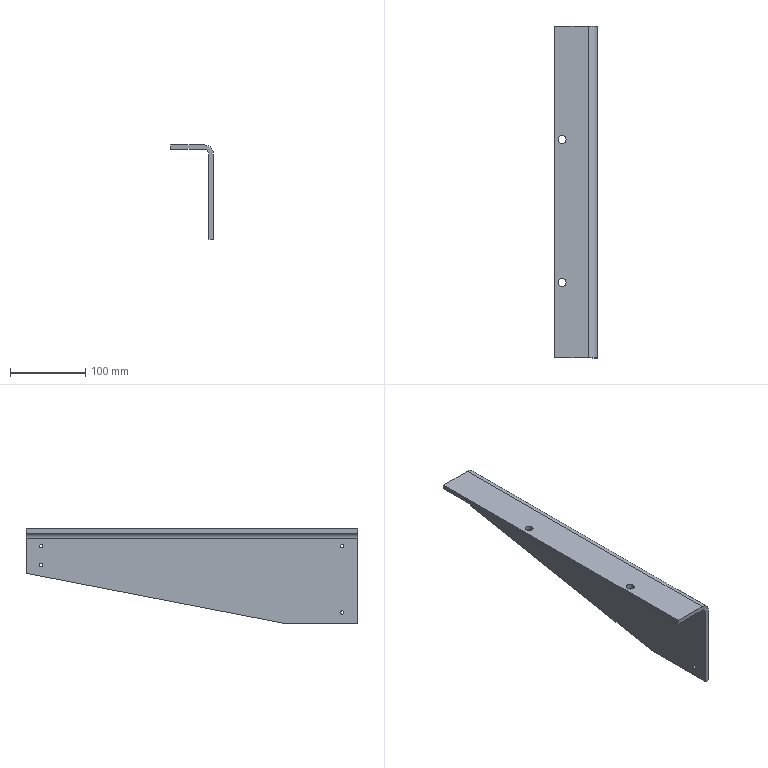Part | NX | features solid 2 | 1 solid | 23 faces | box 57 x 441 x 125 mm | volume 386523 mm3 | cylinder 14 | plane 9 | commonest cylinder face diameters 4.459 x8 10.6 x4 12 x1 24 x1
STEP:
#1=CARTESIAN_POINT('',(-333.,473.229,-255.));
#2=VERTEX_POINT('',#1);
#3=CARTESIAN_POINT('',(-339.,473.229,-255.));
#4=VERTEX_POINT('',#3);
#5=CARTESIAN_POINT('',(-794.904,473.229,-255.));
#6=DIRECTION('',(1.,0.,0.));
#7=VECTOR('',#6,1000.);
#8=LINE('',#5,#7);
#9=EDGE_CURVE('',#2,#4,#8,.F.);
#10=ORIENTED_EDGE('',*,*,#9,.T.);
#11=CARTESIAN_POINT('',(-339.,468.77,-255.));
#12=VERTEX_POINT('',#11);
#13=CARTESIAN_POINT('',(-339.,471.,-255.));
#14=DIRECTION('',(1.,0.,0.));
#15=DIRECTION('',(0.,1.,0.));
#16=AXIS2_PLACEMENT_3D('',#13,#14,#15);
#17=CIRCLE('',#16,2.229);
#18=EDGE_CURVE('',#12,#4,#17,.T.);
#19=ORIENTED_EDGE('',*,*,#18,.F.);
#20=CARTESIAN_POINT('',(-333.,468.77,-255.));
#21=VERTEX_POINT('',#20);
#22=CARTESIAN_POINT('',(-794.904,468.77,-255.));
#23=DIRECTION('',(1.,0.,0.));
#24=VECTOR('',#23,1000.);
#25=LINE('',#22,#24);
#26=EDGE_CURVE('',#12,#21,#25,.T.);
#27=ORIENTED_EDGE('',*,*,#26,.T.);
#28=CARTESIAN_POINT('',(-333.,471.,-255.));
#29=DIRECTION('',(-1.,0.,0.));
#30=DIRECTION('',(0.,-1.,0.));
#31=AXIS2_PLACEMENT_3D('',#28,#29,#30);
#32=CIRCLE('',#31,2.229);
#33=EDGE_CURVE('',#2,#21,#32,.T.);
#34=ORIENTED_EDGE('',*,*,#33,.F.);
#35=EDGE_LOOP('',(#10,#19,#27,#34));
#36=FACE_BOUND('',#35,.T.);
#37=CARTESIAN_POINT('',(-794.904,471.,-255.));
#38=DIRECTION('',(1.,0.,0.));
#39=DIRECTION('',(0.,-1.,0.));
#40=AXIS2_PLACEMENT_3D('',#37,#38,#39);
#41=CYLINDRICAL_SURFACE('',#40,2.229);
#42=ADVANCED_FACE('',(#36),#41,.F.);
#43=CARTESIAN_POINT('',(-333.,473.229,-230.));
#44=VERTEX_POINT('',#43);
#45=CARTESIAN_POINT('',(-339.,473.229,-230.));
#46=VERTEX_POINT('',#45);
#47=CARTESIAN_POINT('',(-794.904,473.229,-230.));
#48=DIRECTION('',(1.,0.,0.));
#49=VECTOR('',#48,1000.);
#50=LINE('',#47,#49);
#51=EDGE_CURVE('',#44,#46,#50,.F.);
#52=ORIENTED_EDGE('',*,*,#51,.T.);
#53=CARTESIAN_POINT('',(-339.,468.77,-230.));
#54=VERTEX_POINT('',#53);
#55=CARTESIAN_POINT('',(-339.,471.,-230.));
#56=DIRECTION('',(1.,0.,0.));
#57=DIRECTION('',(0.,1.,0.));
#58=AXIS2_PLACEMENT_3D('',#55,#56,#57);
#59=CIRCLE('',#58,2.229);
#60=EDGE_CURVE('',#54,#46,#59,.T.);
#61=ORIENTED_EDGE('',*,*,#60,.F.);
#62=CARTESIAN_POINT('',(-333.,468.77,-230.));
#63=VERTEX_POINT('',#62);
#64=CARTESIAN_POINT('',(-794.904,468.77,-230.));
#65=DIRECTION('',(1.,0.,0.));
#66=VECTOR('',#65,1000.);
#67=LINE('',#64,#66);
#68=EDGE_CURVE('',#54,#63,#67,.T.);
#69=ORIENTED_EDGE('',*,*,#68,.T.);
#70=CARTESIAN_POINT('',(-333.,471.,-230.));
#71=DIRECTION('',(-1.,0.,0.));
#72=DIRECTION('',(0.,-1.,0.));
#73=AXIS2_PLACEMENT_3D('',#70,#71,#72);
#74=CIRCLE('',#73,2.229);
#75=EDGE_CURVE('',#44,#63,#74,.T.);
#76=ORIENTED_EDGE('',*,*,#75,.F.);
#77=EDGE_LOOP('',(#52,#61,#69,#76));
#78=FACE_BOUND('',#77,.T.);
#79=CARTESIAN_POINT('',(-794.904,471.,-230.));
#80=DIRECTION('',(1.,0.,0.));
#81=DIRECTION('',(0.,-1.,0.));
#82=AXIS2_PLACEMENT_3D('',#79,#80,#81);
#83=CYLINDRICAL_SURFACE('',#82,2.229);
#84=ADVANCED_FACE('',(#78),#83,.F.);
#85=CARTESIAN_POINT('',(-333.,73.23,-318.));
#86=VERTEX_POINT('',#85);
#87=CARTESIAN_POINT('',(-339.,73.23,-318.));
#88=VERTEX_POINT('',#87);
#89=CARTESIAN_POINT('',(-794.904,73.23,-318.));
#90=DIRECTION('',(1.,0.,0.));
#91=VECTOR('',#90,1000.);
#92=LINE('',#89,#91);
#93=EDGE_CURVE('',#86,#88,#92,.F.);
#94=ORIENTED_EDGE('',*,*,#93,.T.);
#95=CARTESIAN_POINT('',(-339.,68.771,-318.));
#96=VERTEX_POINT('',#95);
#97=CARTESIAN_POINT('',(-339.,71.,-318.));
#98=DIRECTION('',(1.,0.,0.));
#99=DIRECTION('',(0.,1.,0.));
#100=AXIS2_PLACEMENT_3D('',#97,#98,#99);
#101=CIRCLE('',#100,2.229);
#102=EDGE_CURVE('',#96,#88,#101,.T.);
#103=ORIENTED_EDGE('',*,*,#102,.F.);
#104=CARTESIAN_POINT('',(-333.,68.771,-318.));
#105=VERTEX_POINT('',#104);
#106=CARTESIAN_POINT('',(-794.904,68.771,-318.));
#107=DIRECTION('',(1.,0.,0.));
#108=VECTOR('',#107,1000.);
#109=LINE('',#106,#108);
#110=EDGE_CURVE('',#96,#105,#109,.T.);
#111=ORIENTED_EDGE('',*,*,#110,.T.);
#112=CARTESIAN_POINT('',(-333.,71.,-318.));
#113=DIRECTION('',(-1.,0.,0.));
#114=DIRECTION('',(0.,-1.,0.));
#115=AXIS2_PLACEMENT_3D('',#112,#113,#114);
#116=CIRCLE('',#115,2.229);
#117=EDGE_CURVE('',#86,#105,#116,.T.);
#118=ORIENTED_EDGE('',*,*,#117,.F.);
#119=EDGE_LOOP('',(#94,#103,#111,#118));
#120=FACE_BOUND('',#119,.T.);
#121=CARTESIAN_POINT('',(-794.904,71.,-318.));
#122=DIRECTION('',(1.,0.,0.));
#123=DIRECTION('',(0.,-1.,0.));
#124=AXIS2_PLACEMENT_3D('',#121,#122,#123);
#125=CYLINDRICAL_SURFACE('',#124,2.229);
#126=ADVANCED_FACE('',(#120),#125,.F.);
#127=CARTESIAN_POINT('',(-333.,73.23,-230.));
#128=VERTEX_POINT('',#127);
#129=CARTESIAN_POINT('',(-339.,73.23,-230.));
#130=VERTEX_POINT('',#129);
#131=CARTESIAN_POINT('',(-794.904,73.23,-230.));
#132=DIRECTION('',(1.,0.,0.));
#133=VECTOR('',#132,1000.);
#134=LINE('',#131,#133);
#135=EDGE_CURVE('',#128,#130,#134,.F.);
#136=ORIENTED_EDGE('',*,*,#135,.T.);
#137=CARTESIAN_POINT('',(-339.,68.771,-230.));
#138=VERTEX_POINT('',#137);
#139=CARTESIAN_POINT('',(-339.,71.,-230.));
#140=DIRECTION('',(1.,0.,0.));
#141=DIRECTION('',(0.,1.,0.));
#142=AXIS2_PLACEMENT_3D('',#139,#140,#141);
#143=CIRCLE('',#142,2.229);
#144=EDGE_CURVE('',#138,#130,#143,.T.);
#145=ORIENTED_EDGE('',*,*,#144,.F.);
#146=CARTESIAN_POINT('',(-333.,68.771,-230.));
#147=VERTEX_POINT('',#146);
#148=CARTESIAN_POINT('',(-794.904,68.771,-230.));
#149=DIRECTION('',(1.,0.,0.));
#150=VECTOR('',#149,1000.);
#151=LINE('',#148,#150);
#152=EDGE_CURVE('',#138,#147,#151,.T.);
#153=ORIENTED_EDGE('',*,*,#152,.T.);
#154=CARTESIAN_POINT('',(-333.,71.,-230.));
#155=DIRECTION('',(-1.,0.,0.));
#156=DIRECTION('',(0.,-1.,0.));
#157=AXIS2_PLACEMENT_3D('',#154,#155,#156);
#158=CIRCLE('',#157,2.229);
#159=EDGE_CURVE('',#128,#147,#158,.T.);
#160=ORIENTED_EDGE('',*,*,#159,.F.);
#161=EDGE_LOOP('',(#136,#145,#153,#160));
#162=FACE_BOUND('',#161,.T.);
#163=CARTESIAN_POINT('',(-794.904,71.,-230.));
#164=DIRECTION('',(1.,0.,0.));
#165=DIRECTION('',(0.,-1.,0.));
#166=AXIS2_PLACEMENT_3D('',#163,#164,#165);
#167=CYLINDRICAL_SURFACE('',#166,2.229);
#168=ADVANCED_FACE('',(#162),#167,.F.);
#169=CARTESIAN_POINT('',(-374.7,340.,-207.));
#170=VERTEX_POINT('',#169);
#171=CARTESIAN_POINT('',(-374.7,340.,-213.));
#172=VERTEX_POINT('',#171);
#173=CARTESIAN_POINT('',(-374.7,340.,-668.904));
#174=DIRECTION('',(0.,0.,1.));
#175=VECTOR('',#174,1000.);
#176=LINE('',#173,#175);
#177=EDGE_CURVE('',#170,#172,#176,.F.);
#178=ORIENTED_EDGE('',*,*,#177,.T.);
#179=CARTESIAN_POINT('',(-385.3,340.,-213.));
#180=VERTEX_POINT('',#179);
#181=CARTESIAN_POINT('',(-380.,340.,-213.));
#182=DIRECTION('',(0.,0.,-1.));
#183=DIRECTION('',(-1.,0.,0.));
#184=AXIS2_PLACEMENT_3D('',#181,#182,#183);
#185=CIRCLE('',#184,5.3);
#186=EDGE_CURVE('',#172,#180,#185,.T.);
#187=ORIENTED_EDGE('',*,*,#186,.T.);
#188=CARTESIAN_POINT('',(-385.3,340.,-207.));
#189=VERTEX_POINT('',#188);
#190=CARTESIAN_POINT('',(-385.3,340.,-668.904));
#191=DIRECTION('',(0.,0.,1.));
#192=VECTOR('',#191,1000.);
#193=LINE('',#190,#192);
#194=EDGE_CURVE('',#180,#189,#193,.T.);
#195=ORIENTED_EDGE('',*,*,#194,.T.);
#196=CARTESIAN_POINT('',(-380.,340.,-207.));
#197=DIRECTION('',(0.,0.,-1.));
#198=DIRECTION('',(0.,-1.,0.));
#199=AXIS2_PLACEMENT_3D('',#196,#197,#198);
#200=CIRCLE('',#199,5.3);
#201=EDGE_CURVE('',#170,#189,#200,.T.);
#202=ORIENTED_EDGE('',*,*,#201,.F.);
#203=EDGE_LOOP('',(#178,#187,#195,#202));
#204=FACE_BOUND('',#203,.T.);
#205=CARTESIAN_POINT('',(-380.,340.,-668.904));
#206=DIRECTION('',(0.,0.,1.));
#207=DIRECTION('',(-1.,0.,0.));
#208=AXIS2_PLACEMENT_3D('',#205,#206,#207);
#209=CYLINDRICAL_SURFACE('',#208,5.3);
#210=ADVANCED_FACE('',(#204),#209,.F.);
#211=CARTESIAN_POINT('',(-374.7,150.,-213.));
#212=VERTEX_POINT('',#211);
#213=CARTESIAN_POINT('',(-374.7,150.,-207.));
#214=VERTEX_POINT('',#213);
#215=CARTESIAN_POINT('',(-374.7,150.,-668.904));
#216=DIRECTION('',(0.,0.,1.));
#217=VECTOR('',#216,1000.);
#218=LINE('',#215,#217);
#219=EDGE_CURVE('',#212,#214,#218,.T.);
#220=ORIENTED_EDGE('',*,*,#219,.F.);
#221=CARTESIAN_POINT('',(-385.3,150.,-213.));
#222=VERTEX_POINT('',#221);
#223=CARTESIAN_POINT('',(-380.,150.,-213.));
#224=DIRECTION('',(0.,0.,-1.));
#225=DIRECTION('',(-1.,0.,0.));
#226=AXIS2_PLACEMENT_3D('',#223,#224,#225);
#227=CIRCLE('',#226,5.3);
#228=EDGE_CURVE('',#212,#222,#227,.T.);
#229=ORIENTED_EDGE('',*,*,#228,.T.);
#230=CARTESIAN_POINT('',(-385.3,150.,-207.));
#231=VERTEX_POINT('',#230);
#232=CARTESIAN_POINT('',(-385.3,150.,-668.904));
#233=DIRECTION('',(0.,0.,1.));
#234=VECTOR('',#233,1000.);
#235=LINE('',#232,#234);
#236=EDGE_CURVE('',#231,#222,#235,.F.);
#237=ORIENTED_EDGE('',*,*,#236,.F.);
#238=CARTESIAN_POINT('',(-380.,150.,-207.));
#239=DIRECTION('',(0.,0.,-1.));
#240=DIRECTION('',(0.,-1.,0.));
#241=AXIS2_PLACEMENT_3D('',#238,#239,#240);
#242=CIRCLE('',#241,5.3);
#243=EDGE_CURVE('',#214,#231,#242,.T.);
#244=ORIENTED_EDGE('',*,*,#243,.F.);
#245=EDGE_LOOP('',(#220,#229,#237,#244));
#246=FACE_BOUND('',#245,.T.);
#247=CARTESIAN_POINT('',(-380.,150.,-668.904));
#248=DIRECTION('',(0.,0.,1.));
#249=DIRECTION('',(-1.,0.,0.));
#250=AXIS2_PLACEMENT_3D('',#247,#248,#249);
#251=CYLINDRICAL_SURFACE('',#250,5.3);
#252=ADVANCED_FACE('',(#246),#251,.F.);
#253=CARTESIAN_POINT('',(-339.,50.,-219.));
#254=VERTEX_POINT('',#253);
#255=CARTESIAN_POINT('',(-339.,491.,-219.));
#256=VERTEX_POINT('',#255);
#257=CARTESIAN_POINT('',(-339.,50.,-219.));
#258=DIRECTION('',(0.,1.,0.));
#259=VECTOR('',#258,1000.);
#260=LINE('',#257,#259);
#261=EDGE_CURVE('',#254,#256,#260,.T.);
#262=ORIENTED_EDGE('',*,*,#261,.F.);
#263=CARTESIAN_POINT('',(-345.,50.,-213.));
#264=VERTEX_POINT('',#263);
#265=CARTESIAN_POINT('',(-345.,50.,-219.));
#266=DIRECTION('',(0.,1.,0.));
#267=DIRECTION('',(1.,0.,0.));
#268=AXIS2_PLACEMENT_3D('',#265,#266,#267);
#269=CIRCLE('',#268,6.);
#270=EDGE_CURVE('',#264,#254,#269,.T.);
#271=ORIENTED_EDGE('',*,*,#270,.F.);
#272=CARTESIAN_POINT('',(-345.,491.,-213.));
#273=VERTEX_POINT('',#272);
#274=CARTESIAN_POINT('',(-345.,491.,-213.));
#275=DIRECTION('',(0.,-1.,0.));
#276=VECTOR('',#275,1000.);
#277=LINE('',#274,#276);
#278=EDGE_CURVE('',#273,#264,#277,.T.);
#279=ORIENTED_EDGE('',*,*,#278,.F.);
#280=CARTESIAN_POINT('',(-345.,491.,-219.));
#281=DIRECTION('',(0.,-1.,0.));
#282=DIRECTION('',(1.,0.,0.));
#283=AXIS2_PLACEMENT_3D('',#280,#281,#282);
#284=CIRCLE('',#283,6.);
#285=EDGE_CURVE('',#256,#273,#284,.T.);
#286=ORIENTED_EDGE('',*,*,#285,.F.);
#287=EDGE_LOOP('',(#262,#271,#279,#286));
#288=FACE_BOUND('',#287,.T.);
#289=CARTESIAN_POINT('',(-345.,50.,-219.));
#290=DIRECTION('',(0.,1.,0.));
#291=DIRECTION('',(-1.,0.,0.));
#292=AXIS2_PLACEMENT_3D('',#289,#290,#291);
#293=CYLINDRICAL_SURFACE('',#292,6.);
#294=ADVANCED_FACE('',(#288),#293,.F.);
#295=CARTESIAN_POINT('',(-333.,50.,-219.));
#296=VERTEX_POINT('',#295);
#297=CARTESIAN_POINT('',(-333.,491.,-219.));
#298=VERTEX_POINT('',#297);
#299=CARTESIAN_POINT('',(-333.,50.,-219.));
#300=DIRECTION('',(0.,1.,0.));
#301=VECTOR('',#300,1000.);
#302=LINE('',#299,#301);
#303=EDGE_CURVE('',#296,#298,#302,.T.);
#304=ORIENTED_EDGE('',*,*,#303,.T.);
#305=CARTESIAN_POINT('',(-345.,491.,-207.));
#306=VERTEX_POINT('',#305);
#307=CARTESIAN_POINT('',(-345.,491.,-219.));
#308=DIRECTION('',(0.,-1.,0.));
#309=DIRECTION('',(-1.,0.,0.));
#310=AXIS2_PLACEMENT_3D('',#307,#308,#309);
#311=CIRCLE('',#310,12.);
#312=EDGE_CURVE('',#298,#306,#311,.T.);
#313=ORIENTED_EDGE('',*,*,#312,.T.);
#314=CARTESIAN_POINT('',(-345.,50.,-207.));
#315=VERTEX_POINT('',#314);
#316=CARTESIAN_POINT('',(-345.,491.,-207.));
#317=DIRECTION('',(0.,-1.,0.));
#318=VECTOR('',#317,1000.);
#319=LINE('',#316,#318);
#320=EDGE_CURVE('',#306,#315,#319,.T.);
#321=ORIENTED_EDGE('',*,*,#320,.T.);
#322=CARTESIAN_POINT('',(-345.,50.,-219.));
#323=DIRECTION('',(0.,1.,0.));
#324=DIRECTION('',(-1.,0.,0.));
#325=AXIS2_PLACEMENT_3D('',#322,#323,#324);
#326=CIRCLE('',#325,12.);
#327=EDGE_CURVE('',#315,#296,#326,.T.);
#328=ORIENTED_EDGE('',*,*,#327,.T.);
#329=EDGE_LOOP('',(#304,#313,#321,#328));
#330=FACE_BOUND('',#329,.T.);
#331=CARTESIAN_POINT('',(-345.,50.,-219.));
#332=DIRECTION('',(0.,1.,0.));
#333=DIRECTION('',(-1.,0.,0.));
#334=AXIS2_PLACEMENT_3D('',#331,#332,#333);
#335=CYLINDRICAL_SURFACE('',#334,12.);
#336=ADVANCED_FACE('',(#330),#335,.T.);
#337=CARTESIAN_POINT('',(-390.,50.,-213.));
#338=VERTEX_POINT('',#337);
#339=CARTESIAN_POINT('',(-390.,491.,-213.));
#340=VERTEX_POINT('',#339);
#341=CARTESIAN_POINT('',(-390.,50.,-213.));
#342=DIRECTION('',(0.,1.,0.));
#343=VECTOR('',#342,1000.);
#344=LINE('',#341,#343);
#345=EDGE_CURVE('',#338,#340,#344,.T.);
#346=ORIENTED_EDGE('',*,*,#345,.F.);
#347=CARTESIAN_POINT('',(-390.,50.,-207.));
#348=VERTEX_POINT('',#347);
#349=CARTESIAN_POINT('',(-390.,50.,-207.));
#350=DIRECTION('',(0.,0.,-1.));
#351=VECTOR('',#350,1000.);
#352=LINE('',#349,#351);
#353=EDGE_CURVE('',#348,#338,#352,.T.);
#354=ORIENTED_EDGE('',*,*,#353,.F.);
#355=CARTESIAN_POINT('',(-390.,491.,-207.));
#356=VERTEX_POINT('',#355);
#357=CARTESIAN_POINT('',(-390.,50.,-207.));
#358=DIRECTION('',(0.,1.,0.));
#359=VECTOR('',#358,1000.);
#360=LINE('',#357,#359);
#361=EDGE_CURVE('',#348,#356,#360,.T.);
#362=ORIENTED_EDGE('',*,*,#361,.T.);
#363=CARTESIAN_POINT('',(-390.,491.,-207.));
#364=DIRECTION('',(0.,0.,-1.));
#365=VECTOR('',#364,1000.);
#366=LINE('',#363,#365);
#367=EDGE_CURVE('',#356,#340,#366,.T.);
#368=ORIENTED_EDGE('',*,*,#367,.T.);
#369=EDGE_LOOP('',(#346,#354,#362,#368));
#370=FACE_BOUND('',#369,.T.);
#371=CARTESIAN_POINT('',(-390.,50.,-207.));
#372=DIRECTION('',(1.,0.,0.));
#373=DIRECTION('',(0.,-1.,0.));
#374=AXIS2_PLACEMENT_3D('',#371,#372,#373);
#375=PLANE('',#374);
#376=ADVANCED_FACE('',(#370),#375,.F.);
#377=CARTESIAN_POINT('',(-380.,150.,-213.));
#378=DIRECTION('',(0.,0.,-1.));
#379=DIRECTION('',(-1.,0.,0.));
#380=AXIS2_PLACEMENT_3D('',#377,#378,#379);
#381=CIRCLE('',#380,5.3);
#382=EDGE_CURVE('',#222,#212,#381,.T.);
#383=ORIENTED_EDGE('',*,*,#382,.F.);
#384=ORIENTED_EDGE('',*,*,#228,.F.);
#385=EDGE_LOOP('',(#383,#384));
#386=FACE_BOUND('',#385,.T.);
#387=CARTESIAN_POINT('',(-380.,340.,-213.));
#388=DIRECTION('',(0.,0.,-1.));
#389=DIRECTION('',(-1.,0.,0.));
#390=AXIS2_PLACEMENT_3D('',#387,#388,#389);
#391=CIRCLE('',#390,5.3);
#392=EDGE_CURVE('',#180,#172,#391,.T.);
#393=ORIENTED_EDGE('',*,*,#392,.F.);
#394=ORIENTED_EDGE('',*,*,#186,.F.);
#395=EDGE_LOOP('',(#393,#394));
#396=FACE_BOUND('',#395,.T.);
#397=ORIENTED_EDGE('',*,*,#278,.T.);
#398=CARTESIAN_POINT('',(-337.931,50.,-213.));
#399=DIRECTION('',(-1.,0.,0.));
#400=VECTOR('',#399,1000.);
#401=LINE('',#398,#400);
#402=EDGE_CURVE('',#264,#338,#401,.T.);
#403=ORIENTED_EDGE('',*,*,#402,.T.);
#404=ORIENTED_EDGE('',*,*,#345,.T.);
#405=CARTESIAN_POINT('',(-337.931,491.,-213.));
#406=DIRECTION('',(1.,0.,0.));
#407=VECTOR('',#406,1000.);
#408=LINE('',#405,#407);
#409=EDGE_CURVE('',#340,#273,#408,.T.);
#410=ORIENTED_EDGE('',*,*,#409,.T.);
#411=EDGE_LOOP('',(#397,#403,#404,#410));
#412=FACE_BOUND('',#411,.T.);
#413=CARTESIAN_POINT('',(-339.,59.94,-213.));
#414=DIRECTION('',(0.,0.,1.));
#415=DIRECTION('',(0.,-1.,0.));
#416=AXIS2_PLACEMENT_3D('',#413,#414,#415);
#417=PLANE('',#416);
#418=ADVANCED_FACE('',(#386,#396,#412),#417,.F.);
#419=CARTESIAN_POINT('',(-380.,150.,-207.));
#420=DIRECTION('',(0.,0.,-1.));
#421=DIRECTION('',(0.,-1.,0.));
#422=AXIS2_PLACEMENT_3D('',#419,#420,#421);
#423=CIRCLE('',#422,5.3);
#424=EDGE_CURVE('',#231,#214,#423,.T.);
#425=ORIENTED_EDGE('',*,*,#424,.T.);
#426=ORIENTED_EDGE('',*,*,#243,.T.);
#427=EDGE_LOOP('',(#425,#426));
#428=FACE_BOUND('',#427,.T.);
#429=CARTESIAN_POINT('',(-380.,340.,-207.));
#430=DIRECTION('',(0.,0.,-1.));
#431=DIRECTION('',(0.,-1.,0.));
#432=AXIS2_PLACEMENT_3D('',#429,#430,#431);
#433=CIRCLE('',#432,5.3);
#434=EDGE_CURVE('',#189,#170,#433,.T.);
#435=ORIENTED_EDGE('',*,*,#434,.T.);
#436=ORIENTED_EDGE('',*,*,#201,.T.);
#437=EDGE_LOOP('',(#435,#436));
#438=FACE_BOUND('',#437,.T.);
#439=CARTESIAN_POINT('',(-337.931,491.,-207.));
#440=DIRECTION('',(1.,0.,0.));
#441=VECTOR('',#440,1000.);
#442=LINE('',#439,#441);
#443=EDGE_CURVE('',#356,#306,#442,.T.);
#444=ORIENTED_EDGE('',*,*,#443,.F.);
#445=ORIENTED_EDGE('',*,*,#361,.F.);
#446=CARTESIAN_POINT('',(-337.931,50.,-207.));
#447=DIRECTION('',(-1.,0.,0.));
#448=VECTOR('',#447,1000.);
#449=LINE('',#446,#448);
#450=EDGE_CURVE('',#315,#348,#449,.T.);
#451=ORIENTED_EDGE('',*,*,#450,.F.);
#452=ORIENTED_EDGE('',*,*,#320,.F.);
#453=EDGE_LOOP('',(#444,#445,#451,#452));
#454=FACE_BOUND('',#453,.T.);
#455=CARTESIAN_POINT('',(-339.,59.94,-207.));
#456=DIRECTION('',(0.,0.,1.));
#457=DIRECTION('',(0.,-1.,0.));
#458=AXIS2_PLACEMENT_3D('',#455,#456,#457);
#459=PLANE('',#458);
#460=ADVANCED_FACE('',(#428,#438,#454),#459,.T.);
#461=ORIENTED_EDGE('',*,*,#144,.T.);
#462=CARTESIAN_POINT('',(-339.,71.,-230.));
#463=DIRECTION('',(1.,0.,0.));
#464=DIRECTION('',(0.,1.,0.));
#465=AXIS2_PLACEMENT_3D('',#462,#463,#464);
#466=CIRCLE('',#465,2.229);
#467=EDGE_CURVE('',#130,#138,#466,.T.);
#468=ORIENTED_EDGE('',*,*,#467,.T.);
#469=EDGE_LOOP('',(#461,#468));
#470=FACE_BOUND('',#469,.T.);
#471=ORIENTED_EDGE('',*,*,#102,.T.);
#472=CARTESIAN_POINT('',(-339.,71.,-318.));
#473=DIRECTION('',(1.,0.,0.));
#474=DIRECTION('',(0.,1.,0.));
#475=AXIS2_PLACEMENT_3D('',#472,#473,#474);
#476=CIRCLE('',#475,2.229);
#477=EDGE_CURVE('',#88,#96,#476,.T.);
#478=ORIENTED_EDGE('',*,*,#477,.T.);
#479=EDGE_LOOP('',(#471,#478));
#480=FACE_BOUND('',#479,.T.);
#481=ORIENTED_EDGE('',*,*,#60,.T.);
#482=CARTESIAN_POINT('',(-339.,471.,-230.));
#483=DIRECTION('',(1.,0.,0.));
#484=DIRECTION('',(0.,1.,0.));
#485=AXIS2_PLACEMENT_3D('',#482,#483,#484);
#486=CIRCLE('',#485,2.229);
#487=EDGE_CURVE('',#46,#54,#486,.T.);
#488=ORIENTED_EDGE('',*,*,#487,.T.);
#489=EDGE_LOOP('',(#481,#488));
#490=FACE_BOUND('',#489,.T.);
#491=ORIENTED_EDGE('',*,*,#18,.T.);
#492=CARTESIAN_POINT('',(-339.,471.,-255.));
#493=DIRECTION('',(1.,0.,0.));
#494=DIRECTION('',(0.,1.,0.));
#495=AXIS2_PLACEMENT_3D('',#492,#493,#494);
#496=CIRCLE('',#495,2.229);
#497=EDGE_CURVE('',#4,#12,#496,.T.);
#498=ORIENTED_EDGE('',*,*,#497,.T.);
#499=EDGE_LOOP('',(#491,#498));
#500=FACE_BOUND('',#499,.T.);
#501=ORIENTED_EDGE('',*,*,#261,.T.);
#502=CARTESIAN_POINT('',(-339.,491.,-266.));
#503=VERTEX_POINT('',#502);
#504=CARTESIAN_POINT('',(-339.,491.,-266.));
#505=DIRECTION('',(0.,0.,1.));
#506=VECTOR('',#505,1000.);
#507=LINE('',#504,#506);
#508=EDGE_CURVE('',#503,#256,#507,.T.);
#509=ORIENTED_EDGE('',*,*,#508,.F.);
#510=CARTESIAN_POINT('',(-339.,150.,-332.));
#511=VERTEX_POINT('',#510);
#512=CARTESIAN_POINT('',(-339.,150.,-332.));
#513=DIRECTION('',(0.,0.9818,0.19));
#514=VECTOR('',#513,1000.);
#515=LINE('',#512,#514);
#516=EDGE_CURVE('',#511,#503,#515,.T.);
#517=ORIENTED_EDGE('',*,*,#516,.F.);
#518=CARTESIAN_POINT('',(-339.,50.,-332.));
#519=VERTEX_POINT('',#518);
#520=CARTESIAN_POINT('',(-339.,50.,-332.));
#521=DIRECTION('',(0.,1.,0.));
#522=VECTOR('',#521,1000.);
#523=LINE('',#520,#522);
#524=EDGE_CURVE('',#519,#511,#523,.T.);
#525=ORIENTED_EDGE('',*,*,#524,.F.);
#526=CARTESIAN_POINT('',(-339.,50.,-207.));
#527=DIRECTION('',(0.,0.,-1.));
#528=VECTOR('',#527,1000.);
#529=LINE('',#526,#528);
#530=EDGE_CURVE('',#254,#519,#529,.T.);
#531=ORIENTED_EDGE('',*,*,#530,.F.);
#532=EDGE_LOOP('',(#501,#509,#517,#525,#531));
#533=FACE_BOUND('',#532,.T.);
#534=CARTESIAN_POINT('',(-339.,59.94,-282.103));
#535=DIRECTION('',(-1.,0.,0.));
#536=DIRECTION('',(0.,0.,1.));
#537=AXIS2_PLACEMENT_3D('',#534,#535,#536);
#538=PLANE('',#537);
#539=ADVANCED_FACE('',(#470,#480,#490,#500,#533),#538,.T.);
#540=ORIENTED_EDGE('',*,*,#516,.T.);
#541=CARTESIAN_POINT('',(-333.,491.,-266.));
#542=VERTEX_POINT('',#541);
#543=CARTESIAN_POINT('',(-333.,491.,-266.));
#544=DIRECTION('',(-1.,0.,0.));
#545=VECTOR('',#544,1000.);
#546=LINE('',#543,#545);
#547=EDGE_CURVE('',#542,#503,#546,.T.);
#548=ORIENTED_EDGE('',*,*,#547,.F.);
#549=CARTESIAN_POINT('',(-333.,150.,-332.));
#550=VERTEX_POINT('',#549);
#551=CARTESIAN_POINT('',(-333.,150.,-332.));
#552=DIRECTION('',(0.,0.9818,0.19));
#553=VECTOR('',#552,1000.);
#554=LINE('',#551,#553);
#555=EDGE_CURVE('',#550,#542,#554,.T.);
#556=ORIENTED_EDGE('',*,*,#555,.F.);
#557=CARTESIAN_POINT('',(-333.,150.,-332.));
#558=DIRECTION('',(-1.,0.,0.));
#559=VECTOR('',#558,1000.);
#560=LINE('',#557,#559);
#561=EDGE_CURVE('',#550,#511,#560,.T.);
#562=ORIENTED_EDGE('',*,*,#561,.T.);
#563=EDGE_LOOP('',(#540,#548,#556,#562));
#564=FACE_BOUND('',#563,.T.);
#565=CARTESIAN_POINT('',(-333.,150.,-332.));
#566=DIRECTION('',(0.,0.19,-0.9818));
#567=DIRECTION('',(-1.,0.,0.));
#568=AXIS2_PLACEMENT_3D('',#565,#566,#567);
#569=PLANE('',#568);
#570=ADVANCED_FACE('',(#564),#569,.T.);
#571=ORIENTED_EDGE('',*,*,#524,.T.);
#572=ORIENTED_EDGE('',*,*,#561,.F.);
#573=CARTESIAN_POINT('',(-333.,50.,-332.));
#574=VERTEX_POINT('',#573);
#575=CARTESIAN_POINT('',(-333.,50.,-332.));
#576=DIRECTION('',(0.,1.,0.));
#577=VECTOR('',#576,1000.);
#578=LINE('',#575,#577);
#579=EDGE_CURVE('',#574,#550,#578,.T.);
#580=ORIENTED_EDGE('',*,*,#579,.F.);
#581=CARTESIAN_POINT('',(-333.,50.,-332.));
#582=DIRECTION('',(-1.,0.,0.));
#583=VECTOR('',#582,1000.);
#584=LINE('',#581,#583);
#585=EDGE_CURVE('',#574,#519,#584,.T.);
#586=ORIENTED_EDGE('',*,*,#585,.T.);
#587=EDGE_LOOP('',(#571,#572,#580,#586));
#588=FACE_BOUND('',#587,.T.);
#589=CARTESIAN_POINT('',(-333.,50.,-332.));
#590=DIRECTION('',(0.,0.,-1.));
#591=DIRECTION('',(-1.,0.,0.));
#592=AXIS2_PLACEMENT_3D('',#589,#590,#591);
#593=PLANE('',#592);
#594=ADVANCED_FACE('',(#588),#593,.T.);
#595=CARTESIAN_POINT('',(-333.,71.,-230.));
#596=DIRECTION('',(-1.,0.,0.));
#597=DIRECTION('',(0.,-1.,0.));
#598=AXIS2_PLACEMENT_3D('',#595,#596,#597);
#599=CIRCLE('',#598,2.229);
#600=EDGE_CURVE('',#147,#128,#599,.T.);
#601=ORIENTED_EDGE('',*,*,#600,.T.);
#602=ORIENTED_EDGE('',*,*,#159,.T.);
#603=EDGE_LOOP('',(#601,#602));
#604=FACE_BOUND('',#603,.T.);
#605=CARTESIAN_POINT('',(-333.,71.,-318.));
#606=DIRECTION('',(-1.,0.,0.));
#607=DIRECTION('',(0.,-1.,0.));
#608=AXIS2_PLACEMENT_3D('',#605,#606,#607);
#609=CIRCLE('',#608,2.229);
#610=EDGE_CURVE('',#105,#86,#609,.T.);
#611=ORIENTED_EDGE('',*,*,#610,.T.);
#612=ORIENTED_EDGE('',*,*,#117,.T.);
#613=EDGE_LOOP('',(#611,#612));
#614=FACE_BOUND('',#613,.T.);
#615=CARTESIAN_POINT('',(-333.,471.,-230.));
#616=DIRECTION('',(-1.,0.,0.));
#617=DIRECTION('',(0.,-1.,0.));
#618=AXIS2_PLACEMENT_3D('',#615,#616,#617);
#619=CIRCLE('',#618,2.229);
#620=EDGE_CURVE('',#63,#44,#619,.T.);
#621=ORIENTED_EDGE('',*,*,#620,.T.);
#622=ORIENTED_EDGE('',*,*,#75,.T.);
#623=EDGE_LOOP('',(#621,#622));
#624=FACE_BOUND('',#623,.T.);
#625=CARTESIAN_POINT('',(-333.,471.,-255.));
#626=DIRECTION('',(-1.,0.,0.));
#627=DIRECTION('',(0.,-1.,0.));
#628=AXIS2_PLACEMENT_3D('',#625,#626,#627);
#629=CIRCLE('',#628,2.229);
#630=EDGE_CURVE('',#21,#2,#629,.T.);
#631=ORIENTED_EDGE('',*,*,#630,.T.);
#632=ORIENTED_EDGE('',*,*,#33,.T.);
#633=EDGE_LOOP('',(#631,#632));
#634=FACE_BOUND('',#633,.T.);
#635=CARTESIAN_POINT('',(-333.,50.,-207.));
#636=DIRECTION('',(0.,0.,-1.));
#637=VECTOR('',#636,1000.);
#638=LINE('',#635,#637);
#639=EDGE_CURVE('',#296,#574,#638,.T.);
#640=ORIENTED_EDGE('',*,*,#639,.T.);
#641=ORIENTED_EDGE('',*,*,#579,.T.);
#642=ORIENTED_EDGE('',*,*,#555,.T.);
#643=CARTESIAN_POINT('',(-333.,491.,-266.));
#644=DIRECTION('',(0.,0.,1.));
#645=VECTOR('',#644,1000.);
#646=LINE('',#643,#645);
#647=EDGE_CURVE('',#542,#298,#646,.T.);
#648=ORIENTED_EDGE('',*,*,#647,.T.);
#649=ORIENTED_EDGE('',*,*,#303,.F.);
#650=EDGE_LOOP('',(#640,#641,#642,#648,#649));
#651=FACE_BOUND('',#650,.T.);
#652=CARTESIAN_POINT('',(-333.,59.94,-282.103));
#653=DIRECTION('',(-1.,0.,0.));
#654=DIRECTION('',(0.,0.,1.));
#655=AXIS2_PLACEMENT_3D('',#652,#653,#654);
#656=PLANE('',#655);
#657=ADVANCED_FACE('',(#604,#614,#624,#634,#651),#656,.F.);
#658=ORIENTED_EDGE('',*,*,#647,.F.);
#659=ORIENTED_EDGE('',*,*,#547,.T.);
#660=ORIENTED_EDGE('',*,*,#508,.T.);
#661=ORIENTED_EDGE('',*,*,#285,.T.);
#662=ORIENTED_EDGE('',*,*,#409,.F.);
#663=ORIENTED_EDGE('',*,*,#367,.F.);
#664=ORIENTED_EDGE('',*,*,#443,.T.);
#665=ORIENTED_EDGE('',*,*,#312,.F.);
#666=EDGE_LOOP('',(#658,#659,#660,#661,#662,#663,#664,#665));
#667=FACE_BOUND('',#666,.T.);
#668=CARTESIAN_POINT('',(-333.,491.,-266.));
#669=DIRECTION('',(0.,1.,0.));
#670=DIRECTION('',(1.,0.,0.));
#671=AXIS2_PLACEMENT_3D('',#668,#669,#670);
#672=PLANE('',#671);
#673=ADVANCED_FACE('',(#667),#672,.T.);
#674=ORIENTED_EDGE('',*,*,#530,.T.);
#675=ORIENTED_EDGE('',*,*,#585,.F.);
#676=ORIENTED_EDGE('',*,*,#639,.F.);
#677=ORIENTED_EDGE('',*,*,#327,.F.);
#678=ORIENTED_EDGE('',*,*,#450,.T.);
#679=ORIENTED_EDGE('',*,*,#353,.T.);
#680=ORIENTED_EDGE('',*,*,#402,.F.);
#681=ORIENTED_EDGE('',*,*,#270,.T.);
#682=EDGE_LOOP('',(#674,#675,#676,#677,#678,#679,#680,#681));
#683=FACE_BOUND('',#682,.T.);
#684=CARTESIAN_POINT('',(-333.,50.,-207.));
#685=DIRECTION('',(0.,-1.,0.));
#686=DIRECTION('',(0.,0.,-1.));
#687=AXIS2_PLACEMENT_3D('',#684,#685,#686);
#688=PLANE('',#687);
#689=ADVANCED_FACE('',(#683),#688,.T.);
#690=ORIENTED_EDGE('',*,*,#382,.T.);
#691=ORIENTED_EDGE('',*,*,#219,.T.);
#692=ORIENTED_EDGE('',*,*,#424,.F.);
#693=ORIENTED_EDGE('',*,*,#236,.T.);
#694=EDGE_LOOP('',(#690,#691,#692,#693));
#695=FACE_BOUND('',#694,.T.);
#696=CARTESIAN_POINT('',(-380.,150.,-668.904));
#697=DIRECTION('',(0.,0.,1.));
#698=DIRECTION('',(-1.,0.,0.));
#699=AXIS2_PLACEMENT_3D('',#696,#697,#698);
#700=CYLINDRICAL_SURFACE('',#699,5.3);
#701=ADVANCED_FACE('',(#695),#700,.F.);
#702=ORIENTED_EDGE('',*,*,#392,.T.);
#703=ORIENTED_EDGE('',*,*,#177,.F.);
#704=ORIENTED_EDGE('',*,*,#434,.F.);
#705=ORIENTED_EDGE('',*,*,#194,.F.);
#706=EDGE_LOOP('',(#702,#703,#704,#705));
#707=FACE_BOUND('',#706,.T.);
#708=CARTESIAN_POINT('',(-380.,340.,-668.904));
#709=DIRECTION('',(0.,0.,1.));
#710=DIRECTION('',(-1.,0.,0.));
#711=AXIS2_PLACEMENT_3D('',#708,#709,#710);
#712=CYLINDRICAL_SURFACE('',#711,5.3);
#713=ADVANCED_FACE('',(#707),#712,.F.);
#714=ORIENTED_EDGE('',*,*,#467,.F.);
#715=ORIENTED_EDGE('',*,*,#135,.F.);
#716=ORIENTED_EDGE('',*,*,#600,.F.);
#717=ORIENTED_EDGE('',*,*,#152,.F.);
#718=EDGE_LOOP('',(#714,#715,#716,#717));
#719=FACE_BOUND('',#718,.T.);
#720=CARTESIAN_POINT('',(-794.904,71.,-230.));
#721=DIRECTION('',(1.,0.,0.));
#722=DIRECTION('',(0.,-1.,0.));
#723=AXIS2_PLACEMENT_3D('',#720,#721,#722);
#724=CYLINDRICAL_SURFACE('',#723,2.229);
#725=ADVANCED_FACE('',(#719),#724,.F.);
#726=ORIENTED_EDGE('',*,*,#477,.F.);
#727=ORIENTED_EDGE('',*,*,#93,.F.);
#728=ORIENTED_EDGE('',*,*,#610,.F.);
#729=ORIENTED_EDGE('',*,*,#110,.F.);
#730=EDGE_LOOP('',(#726,#727,#728,#729));
#731=FACE_BOUND('',#730,.T.);
#732=CARTESIAN_POINT('',(-794.904,71.,-318.));
#733=DIRECTION('',(1.,0.,0.));
#734=DIRECTION('',(0.,-1.,0.));
#735=AXIS2_PLACEMENT_3D('',#732,#733,#734);
#736=CYLINDRICAL_SURFACE('',#735,2.229);
#737=ADVANCED_FACE('',(#731),#736,.F.);
#738=ORIENTED_EDGE('',*,*,#487,.F.);
#739=ORIENTED_EDGE('',*,*,#51,.F.);
#740=ORIENTED_EDGE('',*,*,#620,.F.);
#741=ORIENTED_EDGE('',*,*,#68,.F.);
#742=EDGE_LOOP('',(#738,#739,#740,#741));
#743=FACE_BOUND('',#742,.T.);
#744=CARTESIAN_POINT('',(-794.904,471.,-230.));
#745=DIRECTION('',(1.,0.,0.));
#746=DIRECTION('',(0.,-1.,0.));
#747=AXIS2_PLACEMENT_3D('',#744,#745,#746);
#748=CYLINDRICAL_SURFACE('',#747,2.229);
#749=ADVANCED_FACE('',(#743),#748,.F.);
#750=ORIENTED_EDGE('',*,*,#497,.F.);
#751=ORIENTED_EDGE('',*,*,#9,.F.);
#752=ORIENTED_EDGE('',*,*,#630,.F.);
#753=ORIENTED_EDGE('',*,*,#26,.F.);
#754=EDGE_LOOP('',(#750,#751,#752,#753));
#755=FACE_BOUND('',#754,.T.);
#756=CARTESIAN_POINT('',(-794.904,471.,-255.));
#757=DIRECTION('',(1.,0.,0.));
#758=DIRECTION('',(0.,-1.,0.));
#759=AXIS2_PLACEMENT_3D('',#756,#757,#758);
#760=CYLINDRICAL_SURFACE('',#759,2.229);
#761=ADVANCED_FACE('',(#755),#760,.F.);
#762=CLOSED_SHELL('',(#42,#84,#126,#168,#210,#252,#294,#336,#376,#418,#460,#539,#570,#594,#657,#673,#689,#701,#713,#725,#737,#749,#761));
#763=MANIFOLD_SOLID_BREP('',#762);
#764=(LENGTH_UNIT()NAMED_UNIT(*)SI_UNIT(.MILLI.,.METRE.));
#765=UNCERTAINTY_MEASURE_WITH_UNIT(LENGTH_MEASURE(0.00001),#764,'','');
#766=(NAMED_UNIT(*)PLANE_ANGLE_UNIT()SI_UNIT($,.RADIAN.));
#767=(NAMED_UNIT(*)SI_UNIT($,.STERADIAN.)SOLID_ANGLE_UNIT());
#768=(GEOMETRIC_REPRESENTATION_CONTEXT(3)GLOBAL_UNCERTAINTY_ASSIGNED_CONTEXT((#765))GLOBAL_UNIT_ASSIGNED_CONTEXT((#764,#766,#767))REPRESENTATION_CONTEXT('',''));
#769=ADVANCED_BREP_SHAPE_REPRESENTATION('',(#763),#768);